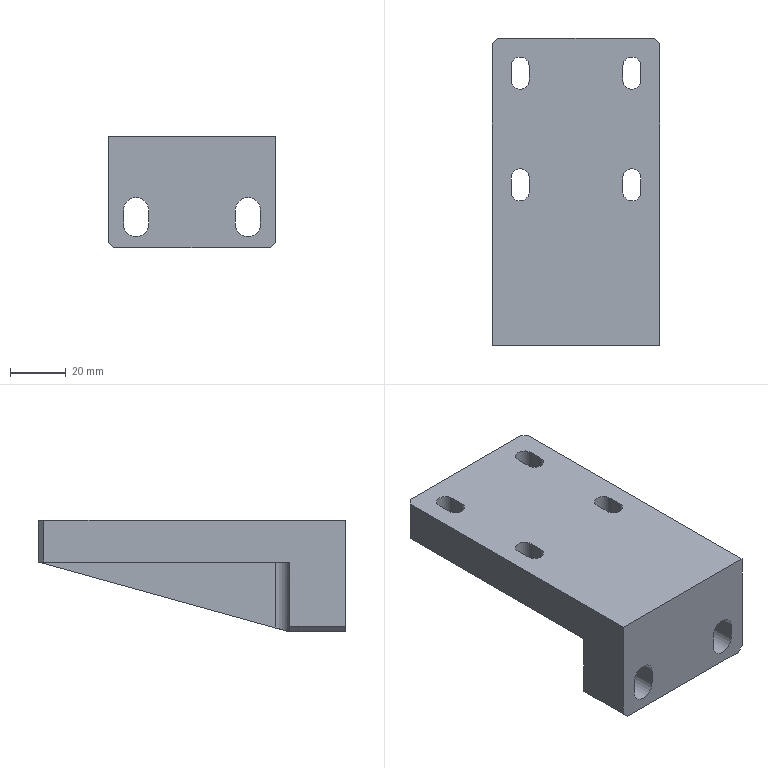Part | STEP file | 1 solid | 65 faces | box 60 x 110 x 40 mm | volume 130636 mm3 | plane 41 | cylinder 24 | commonest cylinder face diameters 6.5 x8 12 x8 9 x6 10 x2